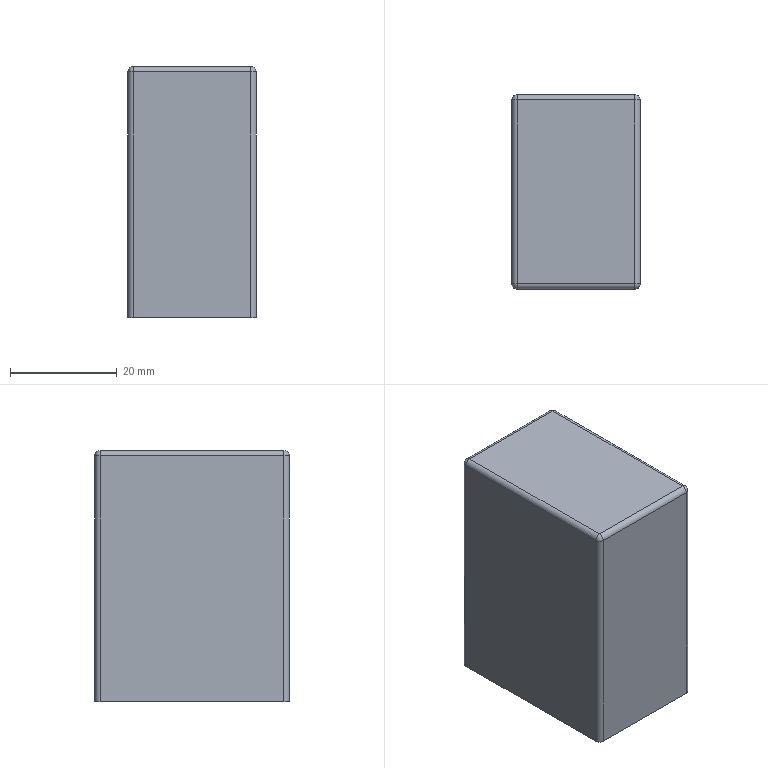Part | NX | features BLEND 3, DATUM_CSYS 2, EXTRUDE 1, SHELL 1, SKETCH 1 | 1 solid | 23 faces | box 24 x 36.4 x 47 mm | volume 6181 mm3 | plane 11 | cylinder 8 | sphere 4 | commonest cylinder face diameters 2 x8
STEP:
#1=CARTESIAN_POINT('',(-12.,-17.2,46.));
#2=VERTEX_POINT('',#1);
#3=CARTESIAN_POINT('',(-12.,17.2,46.));
#4=VERTEX_POINT('',#3);
#5=CARTESIAN_POINT('',(-12.,18.2,46.));
#6=DIRECTION('',(0.,-1.,0.));
#7=VECTOR('',#6,1000.);
#8=LINE('',#5,#7);
#9=EDGE_CURVE('',#2,#4,#8,.F.);
#10=ORIENTED_EDGE('',*,*,#9,.T.);
#11=CARTESIAN_POINT('',(-12.,17.2,0.));
#12=VERTEX_POINT('',#11);
#13=CARTESIAN_POINT('',(-12.,17.2,47.));
#14=DIRECTION('',(0.,0.,-1.));
#15=VECTOR('',#14,1000.);
#16=LINE('',#13,#15);
#17=EDGE_CURVE('',#4,#12,#16,.T.);
#18=ORIENTED_EDGE('',*,*,#17,.T.);
#19=CARTESIAN_POINT('',(-12.,-17.2,0.));
#20=VERTEX_POINT('',#19);
#21=CARTESIAN_POINT('',(-12.,18.2,0.));
#22=DIRECTION('',(0.,-1.,0.));
#23=VECTOR('',#22,1000.);
#24=LINE('',#21,#23);
#25=EDGE_CURVE('',#12,#20,#24,.T.);
#26=ORIENTED_EDGE('',*,*,#25,.T.);
#27=CARTESIAN_POINT('',(-12.,-17.2,47.));
#28=DIRECTION('',(0.,0.,-1.));
#29=VECTOR('',#28,1000.);
#30=LINE('',#27,#29);
#31=EDGE_CURVE('',#20,#2,#30,.F.);
#32=ORIENTED_EDGE('',*,*,#31,.T.);
#33=EDGE_LOOP('',(#10,#18,#26,#32));
#34=FACE_BOUND('',#33,.T.);
#35=CARTESIAN_POINT('',(-12.,18.2,47.));
#36=DIRECTION('',(1.,0.,0.));
#37=DIRECTION('',(0.,1.,0.));
#38=AXIS2_PLACEMENT_3D('',#35,#36,#37);
#39=PLANE('',#38);
#40=ADVANCED_FACE('',(#34),#39,.F.);
#41=CARTESIAN_POINT('',(11.,-18.2,46.));
#42=VERTEX_POINT('',#41);
#43=CARTESIAN_POINT('',(-11.,-18.2,46.));
#44=VERTEX_POINT('',#43);
#45=CARTESIAN_POINT('',(-12.,-18.2,46.));
#46=DIRECTION('',(1.,0.,0.));
#47=VECTOR('',#46,1000.);
#48=LINE('',#45,#47);
#49=EDGE_CURVE('',#42,#44,#48,.F.);
#50=ORIENTED_EDGE('',*,*,#49,.T.);
#51=CARTESIAN_POINT('',(-11.,-18.2,0.));
#52=VERTEX_POINT('',#51);
#53=CARTESIAN_POINT('',(-11.,-18.2,47.));
#54=DIRECTION('',(0.,0.,-1.));
#55=VECTOR('',#54,1000.);
#56=LINE('',#53,#55);
#57=EDGE_CURVE('',#44,#52,#56,.T.);
#58=ORIENTED_EDGE('',*,*,#57,.T.);
#59=CARTESIAN_POINT('',(11.,-18.2,0.));
#60=VERTEX_POINT('',#59);
#61=CARTESIAN_POINT('',(-12.,-18.2,0.));
#62=DIRECTION('',(1.,0.,0.));
#63=VECTOR('',#62,1000.);
#64=LINE('',#61,#63);
#65=EDGE_CURVE('',#52,#60,#64,.T.);
#66=ORIENTED_EDGE('',*,*,#65,.T.);
#67=CARTESIAN_POINT('',(11.,-18.2,47.));
#68=DIRECTION('',(0.,0.,-1.));
#69=VECTOR('',#68,1000.);
#70=LINE('',#67,#69);
#71=EDGE_CURVE('',#60,#42,#70,.F.);
#72=ORIENTED_EDGE('',*,*,#71,.T.);
#73=EDGE_LOOP('',(#50,#58,#66,#72));
#74=FACE_BOUND('',#73,.T.);
#75=CARTESIAN_POINT('',(-12.,-18.2,47.));
#76=DIRECTION('',(0.,1.,0.));
#77=DIRECTION('',(0.,0.,1.));
#78=AXIS2_PLACEMENT_3D('',#75,#76,#77);
#79=PLANE('',#78);
#80=ADVANCED_FACE('',(#74),#79,.F.);
#81=CARTESIAN_POINT('',(12.,-17.2,0.));
#82=VERTEX_POINT('',#81);
#83=CARTESIAN_POINT('',(12.,17.2,0.));
#84=VERTEX_POINT('',#83);
#85=CARTESIAN_POINT('',(12.,-18.2,0.));
#86=DIRECTION('',(0.,1.,0.));
#87=VECTOR('',#86,1000.);
#88=LINE('',#85,#87);
#89=EDGE_CURVE('',#82,#84,#88,.T.);
#90=ORIENTED_EDGE('',*,*,#89,.T.);
#91=CARTESIAN_POINT('',(12.,17.2,46.));
#92=VERTEX_POINT('',#91);
#93=CARTESIAN_POINT('',(12.,17.2,47.));
#94=DIRECTION('',(0.,0.,-1.));
#95=VECTOR('',#94,1000.);
#96=LINE('',#93,#95);
#97=EDGE_CURVE('',#84,#92,#96,.F.);
#98=ORIENTED_EDGE('',*,*,#97,.T.);
#99=CARTESIAN_POINT('',(12.,-17.2,46.));
#100=VERTEX_POINT('',#99);
#101=CARTESIAN_POINT('',(12.,-18.2,46.));
#102=DIRECTION('',(0.,1.,0.));
#103=VECTOR('',#102,1000.);
#104=LINE('',#101,#103);
#105=EDGE_CURVE('',#92,#100,#104,.F.);
#106=ORIENTED_EDGE('',*,*,#105,.T.);
#107=CARTESIAN_POINT('',(12.,-17.2,47.));
#108=DIRECTION('',(0.,0.,-1.));
#109=VECTOR('',#108,1000.);
#110=LINE('',#107,#109);
#111=EDGE_CURVE('',#100,#82,#110,.T.);
#112=ORIENTED_EDGE('',*,*,#111,.T.);
#113=EDGE_LOOP('',(#90,#98,#106,#112));
#114=FACE_BOUND('',#113,.T.);
#115=CARTESIAN_POINT('',(12.,-18.2,47.));
#116=DIRECTION('',(-1.,0.,0.));
#117=DIRECTION('',(0.,-1.,0.));
#118=AXIS2_PLACEMENT_3D('',#115,#116,#117);
#119=PLANE('',#118);
#120=ADVANCED_FACE('',(#114),#119,.F.);
#121=CARTESIAN_POINT('',(11.,18.2,0.));
#122=VERTEX_POINT('',#121);
#123=CARTESIAN_POINT('',(-11.,18.2,0.));
#124=VERTEX_POINT('',#123);
#125=CARTESIAN_POINT('',(12.,18.2,0.));
#126=DIRECTION('',(-1.,0.,0.));
#127=VECTOR('',#126,1000.);
#128=LINE('',#125,#127);
#129=EDGE_CURVE('',#122,#124,#128,.T.);
#130=ORIENTED_EDGE('',*,*,#129,.T.);
#131=CARTESIAN_POINT('',(-11.,18.2,46.));
#132=VERTEX_POINT('',#131);
#133=CARTESIAN_POINT('',(-11.,18.2,47.));
#134=DIRECTION('',(0.,0.,-1.));
#135=VECTOR('',#134,1000.);
#136=LINE('',#133,#135);
#137=EDGE_CURVE('',#124,#132,#136,.F.);
#138=ORIENTED_EDGE('',*,*,#137,.T.);
#139=CARTESIAN_POINT('',(11.,18.2,46.));
#140=VERTEX_POINT('',#139);
#141=CARTESIAN_POINT('',(12.,18.2,46.));
#142=DIRECTION('',(-1.,0.,0.));
#143=VECTOR('',#142,1000.);
#144=LINE('',#141,#143);
#145=EDGE_CURVE('',#132,#140,#144,.F.);
#146=ORIENTED_EDGE('',*,*,#145,.T.);
#147=CARTESIAN_POINT('',(11.,18.2,47.));
#148=DIRECTION('',(0.,0.,-1.));
#149=VECTOR('',#148,1000.);
#150=LINE('',#147,#149);
#151=EDGE_CURVE('',#140,#122,#150,.T.);
#152=ORIENTED_EDGE('',*,*,#151,.T.);
#153=EDGE_LOOP('',(#130,#138,#146,#152));
#154=FACE_BOUND('',#153,.T.);
#155=CARTESIAN_POINT('',(12.,18.2,47.));
#156=DIRECTION('',(0.,-1.,0.));
#157=DIRECTION('',(0.,0.,-1.));
#158=AXIS2_PLACEMENT_3D('',#155,#156,#157);
#159=PLANE('',#158);
#160=ADVANCED_FACE('',(#154),#159,.F.);
#161=CARTESIAN_POINT('',(11.,17.2,47.));
#162=VERTEX_POINT('',#161);
#163=CARTESIAN_POINT('',(-11.,17.2,47.));
#164=VERTEX_POINT('',#163);
#165=CARTESIAN_POINT('',(-12.,17.2,47.));
#166=DIRECTION('',(-1.,0.,0.));
#167=VECTOR('',#166,1000.);
#168=LINE('',#165,#167);
#169=EDGE_CURVE('',#162,#164,#168,.T.);
#170=ORIENTED_EDGE('',*,*,#169,.T.);
#171=CARTESIAN_POINT('',(-11.,-17.2,47.));
#172=VERTEX_POINT('',#171);
#173=CARTESIAN_POINT('',(-11.,-18.2,47.));
#174=DIRECTION('',(0.,-1.,0.));
#175=VECTOR('',#174,1000.);
#176=LINE('',#173,#175);
#177=EDGE_CURVE('',#164,#172,#176,.T.);
#178=ORIENTED_EDGE('',*,*,#177,.T.);
#179=CARTESIAN_POINT('',(11.,-17.2,47.));
#180=VERTEX_POINT('',#179);
#181=CARTESIAN_POINT('',(12.,-17.2,47.));
#182=DIRECTION('',(1.,0.,0.));
#183=VECTOR('',#182,1000.);
#184=LINE('',#181,#183);
#185=EDGE_CURVE('',#172,#180,#184,.T.);
#186=ORIENTED_EDGE('',*,*,#185,.T.);
#187=CARTESIAN_POINT('',(11.,18.2,47.));
#188=DIRECTION('',(0.,1.,0.));
#189=VECTOR('',#188,1000.);
#190=LINE('',#187,#189);
#191=EDGE_CURVE('',#180,#162,#190,.T.);
#192=ORIENTED_EDGE('',*,*,#191,.T.);
#193=EDGE_LOOP('',(#170,#178,#186,#192));
#194=FACE_BOUND('',#193,.T.);
#195=CARTESIAN_POINT('',(0.,0.,47.));
#196=DIRECTION('',(0.,0.,1.));
#197=DIRECTION('',(1.,0.,0.));
#198=AXIS2_PLACEMENT_3D('',#195,#196,#197);
#199=PLANE('',#198);
#200=ADVANCED_FACE('',(#194),#199,.T.);
#201=CARTESIAN_POINT('',(11.,17.2,0.));
#202=VERTEX_POINT('',#201);
#203=CARTESIAN_POINT('',(-11.,17.2,0.));
#204=VERTEX_POINT('',#203);
#205=CARTESIAN_POINT('',(12.,17.2,0.));
#206=DIRECTION('',(-1.,0.,0.));
#207=VECTOR('',#206,1000.);
#208=LINE('',#205,#207);
#209=EDGE_CURVE('',#202,#204,#208,.T.);
#210=ORIENTED_EDGE('',*,*,#209,.T.);
#211=CARTESIAN_POINT('',(-11.,-17.2,0.));
#212=VERTEX_POINT('',#211);
#213=CARTESIAN_POINT('',(-11.,18.2,0.));
#214=DIRECTION('',(0.,-1.,0.));
#215=VECTOR('',#214,1000.);
#216=LINE('',#213,#215);
#217=EDGE_CURVE('',#204,#212,#216,.T.);
#218=ORIENTED_EDGE('',*,*,#217,.T.);
#219=CARTESIAN_POINT('',(11.,-17.2,0.));
#220=VERTEX_POINT('',#219);
#221=CARTESIAN_POINT('',(-12.,-17.2,0.));
#222=DIRECTION('',(1.,0.,0.));
#223=VECTOR('',#222,1000.);
#224=LINE('',#221,#223);
#225=EDGE_CURVE('',#212,#220,#224,.T.);
#226=ORIENTED_EDGE('',*,*,#225,.T.);
#227=CARTESIAN_POINT('',(11.,-18.2,0.));
#228=DIRECTION('',(0.,1.,0.));
#229=VECTOR('',#228,1000.);
#230=LINE('',#227,#229);
#231=EDGE_CURVE('',#220,#202,#230,.T.);
#232=ORIENTED_EDGE('',*,*,#231,.T.);
#233=EDGE_LOOP('',(#210,#218,#226,#232));
#234=FACE_BOUND('',#233,.T.);
#235=ORIENTED_EDGE('',*,*,#25,.F.);
#236=CARTESIAN_POINT('',(-11.,17.2,0.));
#237=DIRECTION('',(0.,0.,1.));
#238=DIRECTION('',(1.,0.,0.));
#239=AXIS2_PLACEMENT_3D('',#236,#237,#238);
#240=CIRCLE('',#239,1.);
#241=EDGE_CURVE('',#12,#124,#240,.F.);
#242=ORIENTED_EDGE('',*,*,#241,.T.);
#243=ORIENTED_EDGE('',*,*,#129,.F.);
#244=CARTESIAN_POINT('',(11.,17.2,0.));
#245=DIRECTION('',(0.,0.,1.));
#246=DIRECTION('',(1.,0.,0.));
#247=AXIS2_PLACEMENT_3D('',#244,#245,#246);
#248=CIRCLE('',#247,1.);
#249=EDGE_CURVE('',#122,#84,#248,.F.);
#250=ORIENTED_EDGE('',*,*,#249,.T.);
#251=ORIENTED_EDGE('',*,*,#89,.F.);
#252=CARTESIAN_POINT('',(11.,-17.2,0.));
#253=DIRECTION('',(0.,0.,1.));
#254=DIRECTION('',(1.,0.,0.));
#255=AXIS2_PLACEMENT_3D('',#252,#253,#254);
#256=CIRCLE('',#255,1.);
#257=EDGE_CURVE('',#82,#60,#256,.F.);
#258=ORIENTED_EDGE('',*,*,#257,.T.);
#259=ORIENTED_EDGE('',*,*,#65,.F.);
#260=CARTESIAN_POINT('',(-11.,-17.2,0.));
#261=DIRECTION('',(0.,0.,1.));
#262=DIRECTION('',(1.,0.,0.));
#263=AXIS2_PLACEMENT_3D('',#260,#261,#262);
#264=CIRCLE('',#263,1.);
#265=EDGE_CURVE('',#52,#20,#264,.F.);
#266=ORIENTED_EDGE('',*,*,#265,.T.);
#267=EDGE_LOOP('',(#235,#242,#243,#250,#251,#258,#259,#266));
#268=FACE_BOUND('',#267,.T.);
#269=CARTESIAN_POINT('',(0.,0.,0.));
#270=DIRECTION('',(0.,0.,1.));
#271=DIRECTION('',(1.,0.,0.));
#272=AXIS2_PLACEMENT_3D('',#269,#270,#271);
#273=PLANE('',#272);
#274=ADVANCED_FACE('',(#234,#268),#273,.F.);
#275=ORIENTED_EDGE('',*,*,#185,.F.);
#276=CARTESIAN_POINT('',(-11.,-17.2,46.));
#277=DIRECTION('',(-1.,0.,0.));
#278=DIRECTION('',(0.,0.,1.));
#279=AXIS2_PLACEMENT_3D('',#276,#277,#278);
#280=CIRCLE('',#279,1.);
#281=EDGE_CURVE('',#172,#44,#280,.F.);
#282=ORIENTED_EDGE('',*,*,#281,.T.);
#283=ORIENTED_EDGE('',*,*,#49,.F.);
#284=CARTESIAN_POINT('',(11.,-17.2,46.));
#285=DIRECTION('',(-1.,0.,0.));
#286=DIRECTION('',(0.,0.,1.));
#287=AXIS2_PLACEMENT_3D('',#284,#285,#286);
#288=CIRCLE('',#287,1.);
#289=EDGE_CURVE('',#42,#180,#288,.T.);
#290=ORIENTED_EDGE('',*,*,#289,.T.);
#291=EDGE_LOOP('',(#275,#282,#283,#290));
#292=FACE_BOUND('',#291,.T.);
#293=CARTESIAN_POINT('',(0.,-17.2,46.));
#294=DIRECTION('',(-1.,0.,0.));
#295=DIRECTION('',(0.,0.,1.));
#296=AXIS2_PLACEMENT_3D('',#293,#294,#295);
#297=CYLINDRICAL_SURFACE('',#296,1.);
#298=ADVANCED_FACE('',(#292),#297,.T.);
#299=ORIENTED_EDGE('',*,*,#105,.F.);
#300=CARTESIAN_POINT('',(11.,17.2,46.));
#301=DIRECTION('',(0.,-1.,0.));
#302=DIRECTION('',(1.,0.,0.));
#303=AXIS2_PLACEMENT_3D('',#300,#301,#302);
#304=CIRCLE('',#303,1.);
#305=EDGE_CURVE('',#92,#162,#304,.T.);
#306=ORIENTED_EDGE('',*,*,#305,.T.);
#307=ORIENTED_EDGE('',*,*,#191,.F.);
#308=CARTESIAN_POINT('',(11.,-17.2,46.));
#309=DIRECTION('',(0.,-1.,0.));
#310=DIRECTION('',(1.,0.,0.));
#311=AXIS2_PLACEMENT_3D('',#308,#309,#310);
#312=CIRCLE('',#311,1.);
#313=EDGE_CURVE('',#180,#100,#312,.F.);
#314=ORIENTED_EDGE('',*,*,#313,.T.);
#315=EDGE_LOOP('',(#299,#306,#307,#314));
#316=FACE_BOUND('',#315,.T.);
#317=CARTESIAN_POINT('',(11.,0.,46.));
#318=DIRECTION('',(0.,-1.,0.));
#319=DIRECTION('',(1.,0.,0.));
#320=AXIS2_PLACEMENT_3D('',#317,#318,#319);
#321=CYLINDRICAL_SURFACE('',#320,1.);
#322=ADVANCED_FACE('',(#316),#321,.T.);
#323=ORIENTED_EDGE('',*,*,#177,.F.);
#324=CARTESIAN_POINT('',(-11.,17.2,46.));
#325=DIRECTION('',(0.,1.,0.));
#326=DIRECTION('',(-1.,0.,0.));
#327=AXIS2_PLACEMENT_3D('',#324,#325,#326);
#328=CIRCLE('',#327,1.);
#329=EDGE_CURVE('',#164,#4,#328,.F.);
#330=ORIENTED_EDGE('',*,*,#329,.T.);
#331=ORIENTED_EDGE('',*,*,#9,.F.);
#332=CARTESIAN_POINT('',(-11.,-17.2,46.));
#333=DIRECTION('',(0.,1.,0.));
#334=DIRECTION('',(-1.,0.,0.));
#335=AXIS2_PLACEMENT_3D('',#332,#333,#334);
#336=CIRCLE('',#335,1.);
#337=EDGE_CURVE('',#2,#172,#336,.T.);
#338=ORIENTED_EDGE('',*,*,#337,.T.);
#339=EDGE_LOOP('',(#323,#330,#331,#338));
#340=FACE_BOUND('',#339,.T.);
#341=CARTESIAN_POINT('',(-11.,0.,46.));
#342=DIRECTION('',(0.,1.,0.));
#343=DIRECTION('',(-1.,0.,0.));
#344=AXIS2_PLACEMENT_3D('',#341,#342,#343);
#345=CYLINDRICAL_SURFACE('',#344,1.);
#346=ADVANCED_FACE('',(#340),#345,.T.);
#347=ORIENTED_EDGE('',*,*,#145,.F.);
#348=CARTESIAN_POINT('',(-11.,17.2,46.));
#349=DIRECTION('',(1.,0.,0.));
#350=DIRECTION('',(0.,0.,-1.));
#351=AXIS2_PLACEMENT_3D('',#348,#349,#350);
#352=CIRCLE('',#351,1.);
#353=EDGE_CURVE('',#132,#164,#352,.T.);
#354=ORIENTED_EDGE('',*,*,#353,.T.);
#355=ORIENTED_EDGE('',*,*,#169,.F.);
#356=CARTESIAN_POINT('',(11.,17.2,46.));
#357=DIRECTION('',(1.,0.,0.));
#358=DIRECTION('',(0.,0.,-1.));
#359=AXIS2_PLACEMENT_3D('',#356,#357,#358);
#360=CIRCLE('',#359,1.);
#361=EDGE_CURVE('',#162,#140,#360,.F.);
#362=ORIENTED_EDGE('',*,*,#361,.T.);
#363=EDGE_LOOP('',(#347,#354,#355,#362));
#364=FACE_BOUND('',#363,.T.);
#365=CARTESIAN_POINT('',(0.,17.2,46.));
#366=DIRECTION('',(1.,0.,0.));
#367=DIRECTION('',(0.,0.,-1.));
#368=AXIS2_PLACEMENT_3D('',#365,#366,#367);
#369=CYLINDRICAL_SURFACE('',#368,1.);
#370=ADVANCED_FACE('',(#364),#369,.T.);
#371=ORIENTED_EDGE('',*,*,#265,.F.);
#372=ORIENTED_EDGE('',*,*,#57,.F.);
#373=CARTESIAN_POINT('',(-11.,-17.2,46.));
#374=DIRECTION('',(0.,0.,1.));
#375=DIRECTION('',(1.,0.,0.));
#376=AXIS2_PLACEMENT_3D('',#373,#374,#375);
#377=CIRCLE('',#376,1.);
#378=EDGE_CURVE('',#2,#44,#377,.T.);
#379=ORIENTED_EDGE('',*,*,#378,.F.);
#380=ORIENTED_EDGE('',*,*,#31,.F.);
#381=EDGE_LOOP('',(#371,#372,#379,#380));
#382=FACE_BOUND('',#381,.T.);
#383=CARTESIAN_POINT('',(-11.,-17.2,47.));
#384=DIRECTION('',(0.,0.,-1.));
#385=DIRECTION('',(-1.,0.,0.));
#386=AXIS2_PLACEMENT_3D('',#383,#384,#385);
#387=CYLINDRICAL_SURFACE('',#386,1.);
#388=ADVANCED_FACE('',(#382),#387,.T.);
#389=ORIENTED_EDGE('',*,*,#378,.T.);
#390=ORIENTED_EDGE('',*,*,#281,.F.);
#391=ORIENTED_EDGE('',*,*,#337,.F.);
#392=EDGE_LOOP('',(#389,#390,#391));
#393=FACE_BOUND('',#392,.T.);
#394=CARTESIAN_POINT('',(-11.,-17.2,46.));
#395=DIRECTION('',(0.,0.,1.));
#396=DIRECTION('',(1.,0.,0.));
#397=AXIS2_PLACEMENT_3D('',#394,#395,#396);
#398=SPHERICAL_SURFACE('',#397,1.);
#399=ADVANCED_FACE('',(#393),#398,.T.);
#400=ORIENTED_EDGE('',*,*,#257,.F.);
#401=ORIENTED_EDGE('',*,*,#111,.F.);
#402=CARTESIAN_POINT('',(11.,-17.2,46.));
#403=DIRECTION('',(0.,0.,1.));
#404=DIRECTION('',(1.,0.,0.));
#405=AXIS2_PLACEMENT_3D('',#402,#403,#404);
#406=CIRCLE('',#405,1.);
#407=EDGE_CURVE('',#42,#100,#406,.T.);
#408=ORIENTED_EDGE('',*,*,#407,.F.);
#409=ORIENTED_EDGE('',*,*,#71,.F.);
#410=EDGE_LOOP('',(#400,#401,#408,#409));
#411=FACE_BOUND('',#410,.T.);
#412=CARTESIAN_POINT('',(11.,-17.2,47.));
#413=DIRECTION('',(0.,0.,-1.));
#414=DIRECTION('',(-1.,0.,0.));
#415=AXIS2_PLACEMENT_3D('',#412,#413,#414);
#416=CYLINDRICAL_SURFACE('',#415,1.);
#417=ADVANCED_FACE('',(#411),#416,.T.);
#418=ORIENTED_EDGE('',*,*,#313,.F.);
#419=ORIENTED_EDGE('',*,*,#289,.F.);
#420=ORIENTED_EDGE('',*,*,#407,.T.);
#421=EDGE_LOOP('',(#418,#419,#420));
#422=FACE_BOUND('',#421,.T.);
#423=CARTESIAN_POINT('',(11.,-17.2,46.));
#424=DIRECTION('',(0.,0.,1.));
#425=DIRECTION('',(1.,0.,0.));
#426=AXIS2_PLACEMENT_3D('',#423,#424,#425);
#427=SPHERICAL_SURFACE('',#426,1.);
#428=ADVANCED_FACE('',(#422),#427,.T.);
#429=ORIENTED_EDGE('',*,*,#241,.F.);
#430=ORIENTED_EDGE('',*,*,#17,.F.);
#431=CARTESIAN_POINT('',(-11.,17.2,46.));
#432=DIRECTION('',(0.,0.,1.));
#433=DIRECTION('',(1.,0.,0.));
#434=AXIS2_PLACEMENT_3D('',#431,#432,#433);
#435=CIRCLE('',#434,1.);
#436=EDGE_CURVE('',#132,#4,#435,.T.);
#437=ORIENTED_EDGE('',*,*,#436,.F.);
#438=ORIENTED_EDGE('',*,*,#137,.F.);
#439=EDGE_LOOP('',(#429,#430,#437,#438));
#440=FACE_BOUND('',#439,.T.);
#441=CARTESIAN_POINT('',(-11.,17.2,47.));
#442=DIRECTION('',(0.,0.,-1.));
#443=DIRECTION('',(-1.,0.,0.));
#444=AXIS2_PLACEMENT_3D('',#441,#442,#443);
#445=CYLINDRICAL_SURFACE('',#444,1.);
#446=ADVANCED_FACE('',(#440),#445,.T.);
#447=ORIENTED_EDGE('',*,*,#436,.T.);
#448=ORIENTED_EDGE('',*,*,#329,.F.);
#449=ORIENTED_EDGE('',*,*,#353,.F.);
#450=EDGE_LOOP('',(#447,#448,#449));
#451=FACE_BOUND('',#450,.T.);
#452=CARTESIAN_POINT('',(-11.,17.2,46.));
#453=DIRECTION('',(0.,0.,1.));
#454=DIRECTION('',(1.,0.,0.));
#455=AXIS2_PLACEMENT_3D('',#452,#453,#454);
#456=SPHERICAL_SURFACE('',#455,1.);
#457=ADVANCED_FACE('',(#451),#456,.T.);
#458=ORIENTED_EDGE('',*,*,#249,.F.);
#459=ORIENTED_EDGE('',*,*,#151,.F.);
#460=CARTESIAN_POINT('',(11.,17.2,46.));
#461=DIRECTION('',(0.,0.,1.));
#462=DIRECTION('',(1.,0.,0.));
#463=AXIS2_PLACEMENT_3D('',#460,#461,#462);
#464=CIRCLE('',#463,1.);
#465=EDGE_CURVE('',#92,#140,#464,.T.);
#466=ORIENTED_EDGE('',*,*,#465,.F.);
#467=ORIENTED_EDGE('',*,*,#97,.F.);
#468=EDGE_LOOP('',(#458,#459,#466,#467));
#469=FACE_BOUND('',#468,.T.);
#470=CARTESIAN_POINT('',(11.,17.2,47.));
#471=DIRECTION('',(0.,0.,-1.));
#472=DIRECTION('',(-1.,0.,0.));
#473=AXIS2_PLACEMENT_3D('',#470,#471,#472);
#474=CYLINDRICAL_SURFACE('',#473,1.);
#475=ADVANCED_FACE('',(#469),#474,.T.);
#476=ORIENTED_EDGE('',*,*,#361,.F.);
#477=ORIENTED_EDGE('',*,*,#305,.F.);
#478=ORIENTED_EDGE('',*,*,#465,.T.);
#479=EDGE_LOOP('',(#476,#477,#478));
#480=FACE_BOUND('',#479,.T.);
#481=CARTESIAN_POINT('',(11.,17.2,46.));
#482=DIRECTION('',(0.,0.,1.));
#483=DIRECTION('',(1.,0.,0.));
#484=AXIS2_PLACEMENT_3D('',#481,#482,#483);
#485=SPHERICAL_SURFACE('',#484,1.);
#486=ADVANCED_FACE('',(#480),#485,.T.);
#487=CARTESIAN_POINT('',(-11.,-17.2,46.));
#488=VERTEX_POINT('',#487);
#489=CARTESIAN_POINT('',(-11.,17.2,46.));
#490=VERTEX_POINT('',#489);
#491=CARTESIAN_POINT('',(-11.,0.,46.));
#492=DIRECTION('',(0.,1.,0.));
#493=VECTOR('',#492,1000.);
#494=LINE('',#491,#493);
#495=EDGE_CURVE('',#488,#490,#494,.T.);
#496=ORIENTED_EDGE('',*,*,#495,.F.);
#497=CARTESIAN_POINT('',(-11.,-17.2,47.));
#498=DIRECTION('',(0.,0.,-1.));
#499=VECTOR('',#498,1000.);
#500=LINE('',#497,#499);
#501=EDGE_CURVE('',#488,#212,#500,.T.);
#502=ORIENTED_EDGE('',*,*,#501,.T.);
#503=ORIENTED_EDGE('',*,*,#217,.F.);
#504=CARTESIAN_POINT('',(-11.,17.2,47.));
#505=DIRECTION('',(0.,0.,-1.));
#506=VECTOR('',#505,1000.);
#507=LINE('',#504,#506);
#508=EDGE_CURVE('',#490,#204,#507,.T.);
#509=ORIENTED_EDGE('',*,*,#508,.F.);
#510=EDGE_LOOP('',(#496,#502,#503,#509));
#511=FACE_BOUND('',#510,.T.);
#512=CARTESIAN_POINT('',(-11.,18.2,47.));
#513=DIRECTION('',(1.,0.,0.));
#514=DIRECTION('',(0.,1.,0.));
#515=AXIS2_PLACEMENT_3D('',#512,#513,#514);
#516=PLANE('',#515);
#517=ADVANCED_FACE('',(#511),#516,.T.);
#518=CARTESIAN_POINT('',(11.,-17.2,46.));
#519=VERTEX_POINT('',#518);
#520=CARTESIAN_POINT('',(0.,-17.2,46.));
#521=DIRECTION('',(-1.,0.,0.));
#522=VECTOR('',#521,1000.);
#523=LINE('',#520,#522);
#524=EDGE_CURVE('',#519,#488,#523,.T.);
#525=ORIENTED_EDGE('',*,*,#524,.F.);
#526=CARTESIAN_POINT('',(11.,-17.2,47.));
#527=DIRECTION('',(0.,0.,-1.));
#528=VECTOR('',#527,1000.);
#529=LINE('',#526,#528);
#530=EDGE_CURVE('',#519,#220,#529,.T.);
#531=ORIENTED_EDGE('',*,*,#530,.T.);
#532=ORIENTED_EDGE('',*,*,#225,.F.);
#533=ORIENTED_EDGE('',*,*,#501,.F.);
#534=EDGE_LOOP('',(#525,#531,#532,#533));
#535=FACE_BOUND('',#534,.T.);
#536=CARTESIAN_POINT('',(-12.,-17.2,47.));
#537=DIRECTION('',(0.,1.,0.));
#538=DIRECTION('',(0.,0.,1.));
#539=AXIS2_PLACEMENT_3D('',#536,#537,#538);
#540=PLANE('',#539);
#541=ADVANCED_FACE('',(#535),#540,.T.);
#542=ORIENTED_EDGE('',*,*,#231,.F.);
#543=ORIENTED_EDGE('',*,*,#530,.F.);
#544=CARTESIAN_POINT('',(11.,17.2,46.));
#545=VERTEX_POINT('',#544);
#546=CARTESIAN_POINT('',(11.,-18.2,46.));
#547=DIRECTION('',(0.,1.,0.));
#548=VECTOR('',#547,1000.);
#549=LINE('',#546,#548);
#550=EDGE_CURVE('',#519,#545,#549,.T.);
#551=ORIENTED_EDGE('',*,*,#550,.T.);
#552=CARTESIAN_POINT('',(11.,17.2,47.));
#553=DIRECTION('',(0.,0.,-1.));
#554=VECTOR('',#553,1000.);
#555=LINE('',#552,#554);
#556=EDGE_CURVE('',#545,#202,#555,.T.);
#557=ORIENTED_EDGE('',*,*,#556,.T.);
#558=EDGE_LOOP('',(#542,#543,#551,#557));
#559=FACE_BOUND('',#558,.T.);
#560=CARTESIAN_POINT('',(11.,-18.2,47.));
#561=DIRECTION('',(-1.,0.,0.));
#562=DIRECTION('',(0.,-1.,0.));
#563=AXIS2_PLACEMENT_3D('',#560,#561,#562);
#564=PLANE('',#563);
#565=ADVANCED_FACE('',(#559),#564,.T.);
#566=ORIENTED_EDGE('',*,*,#209,.F.);
#567=ORIENTED_EDGE('',*,*,#556,.F.);
#568=CARTESIAN_POINT('',(12.,17.2,46.));
#569=DIRECTION('',(-1.,0.,0.));
#570=VECTOR('',#569,1000.);
#571=LINE('',#568,#570);
#572=EDGE_CURVE('',#545,#490,#571,.T.);
#573=ORIENTED_EDGE('',*,*,#572,.T.);
#574=ORIENTED_EDGE('',*,*,#508,.T.);
#575=EDGE_LOOP('',(#566,#567,#573,#574));
#576=FACE_BOUND('',#575,.T.);
#577=CARTESIAN_POINT('',(12.,17.2,47.));
#578=DIRECTION('',(0.,-1.,0.));
#579=DIRECTION('',(0.,0.,-1.));
#580=AXIS2_PLACEMENT_3D('',#577,#578,#579);
#581=PLANE('',#580);
#582=ADVANCED_FACE('',(#576),#581,.T.);
#583=ORIENTED_EDGE('',*,*,#572,.F.);
#584=ORIENTED_EDGE('',*,*,#550,.F.);
#585=ORIENTED_EDGE('',*,*,#524,.T.);
#586=ORIENTED_EDGE('',*,*,#495,.T.);
#587=EDGE_LOOP('',(#583,#584,#585,#586));
#588=FACE_BOUND('',#587,.T.);
#589=CARTESIAN_POINT('',(0.,0.,46.));
#590=DIRECTION('',(0.,0.,1.));
#591=DIRECTION('',(1.,0.,0.));
#592=AXIS2_PLACEMENT_3D('',#589,#590,#591);
#593=PLANE('',#592);
#594=ADVANCED_FACE('',(#588),#593,.F.);
#595=CLOSED_SHELL('',(#40,#80,#120,#160,#200,#274,#298,#322,#346,#370,#388,#399,#417,#428,#446,#457,#475,#486,#517,#541,#565,#582,#594));
#596=MANIFOLD_SOLID_BREP('',#595);
#597=(LENGTH_UNIT()NAMED_UNIT(*)SI_UNIT(.MILLI.,.METRE.));
#598=UNCERTAINTY_MEASURE_WITH_UNIT(LENGTH_MEASURE(0.00001),#597,'','');
#599=(NAMED_UNIT(*)PLANE_ANGLE_UNIT()SI_UNIT($,.RADIAN.));
#600=(NAMED_UNIT(*)SI_UNIT($,.STERADIAN.)SOLID_ANGLE_UNIT());
#601=(GEOMETRIC_REPRESENTATION_CONTEXT(3)GLOBAL_UNCERTAINTY_ASSIGNED_CONTEXT((#598))GLOBAL_UNIT_ASSIGNED_CONTEXT((#597,#599,#600))REPRESENTATION_CONTEXT('',''));
#602=ADVANCED_BREP_SHAPE_REPRESENTATION('',(#596),#601);